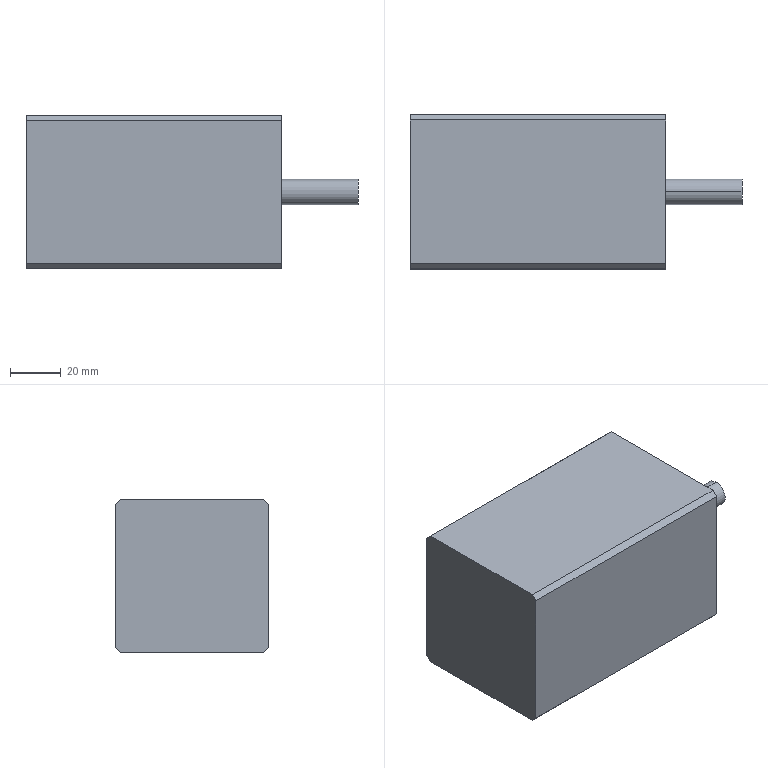Part | STEP file | Guide wheel mechanism revised.sldasm-Part-415 | 1 solid | 13 faces | box 130.5 x 60.5 x 60.5 mm | volume 369407 mm3 | plane 11 | cylinder 2 | commonest cylinder face diameters 10 x2
STEP:
#1=CARTESIAN_POINT('',(130.5,0.,5.));
#2=VERTEX_POINT('',#1);
#3=CARTESIAN_POINT('',(130.5,0.,-5.));
#4=VERTEX_POINT('',#3);
#5=CARTESIAN_POINT('',(130.5,0.,0.));
#6=DIRECTION('',(-1.,0.,0.));
#7=DIRECTION('',(0.,0.,1.));
#8=AXIS2_PLACEMENT_3D('',#5,#6,#7);
#9=CIRCLE('',#8,5.);
#10=EDGE_CURVE('',#2,#4,#9,.T.);
#11=ORIENTED_EDGE('',*,*,#10,.T.);
#12=CARTESIAN_POINT('',(100.5,0.,-5.));
#13=VERTEX_POINT('',#12);
#14=CARTESIAN_POINT('',(130.5,0.,-5.));
#15=DIRECTION('',(-1.,0.,0.));
#16=VECTOR('',#15,1000.);
#17=LINE('',#14,#16);
#18=EDGE_CURVE('',#4,#13,#17,.T.);
#19=ORIENTED_EDGE('',*,*,#18,.T.);
#20=CARTESIAN_POINT('',(100.5,0.,5.));
#21=VERTEX_POINT('',#20);
#22=CARTESIAN_POINT('',(100.5,0.,0.));
#23=DIRECTION('',(-1.,0.,0.));
#24=DIRECTION('',(0.,0.,-1.));
#25=AXIS2_PLACEMENT_3D('',#22,#23,#24);
#26=CIRCLE('',#25,5.);
#27=EDGE_CURVE('',#21,#13,#26,.T.);
#28=ORIENTED_EDGE('',*,*,#27,.F.);
#29=CARTESIAN_POINT('',(130.5,0.,5.));
#30=DIRECTION('',(-1.,0.,0.));
#31=VECTOR('',#30,1000.);
#32=LINE('',#29,#31);
#33=EDGE_CURVE('',#2,#21,#32,.T.);
#34=ORIENTED_EDGE('',*,*,#33,.F.);
#35=EDGE_LOOP('',(#11,#19,#28,#34));
#36=FACE_OUTER_BOUND('',#35,.T.);
#37=CARTESIAN_POINT('',(130.5,0.,0.));
#38=DIRECTION('',(-1.,0.,0.));
#39=DIRECTION('',(0.,0.,1.));
#40=AXIS2_PLACEMENT_3D('',#37,#38,#39);
#41=CYLINDRICAL_SURFACE('',#40,5.);
#42=ADVANCED_FACE('',(#36),#41,.T.);
#43=CARTESIAN_POINT('',(100.5,30.2,28.25));
#44=VERTEX_POINT('',#43);
#45=CARTESIAN_POINT('',(100.5,28.2,30.25));
#46=VERTEX_POINT('',#45);
#47=CARTESIAN_POINT('',(100.5,30.2,28.25));
#48=DIRECTION('',(0.,-0.7071,0.7071));
#49=VECTOR('',#48,1000.);
#50=LINE('',#47,#49);
#51=EDGE_CURVE('',#44,#46,#50,.T.);
#52=ORIENTED_EDGE('',*,*,#51,.T.);
#53=CARTESIAN_POINT('',(100.5,-28.3,30.25));
#54=VERTEX_POINT('',#53);
#55=CARTESIAN_POINT('',(100.5,28.2,30.25));
#56=DIRECTION('',(0.,-1.,0.));
#57=VECTOR('',#56,1000.);
#58=LINE('',#55,#57);
#59=EDGE_CURVE('',#46,#54,#58,.T.);
#60=ORIENTED_EDGE('',*,*,#59,.T.);
#61=CARTESIAN_POINT('',(100.5,-30.3,28.25));
#62=VERTEX_POINT('',#61);
#63=CARTESIAN_POINT('',(100.5,-28.3,30.25));
#64=DIRECTION('',(0.,-0.7071,-0.7071));
#65=VECTOR('',#64,1000.);
#66=LINE('',#63,#65);
#67=EDGE_CURVE('',#54,#62,#66,.T.);
#68=ORIENTED_EDGE('',*,*,#67,.T.);
#69=CARTESIAN_POINT('',(100.5,-30.3,-28.25));
#70=VERTEX_POINT('',#69);
#71=CARTESIAN_POINT('',(100.5,-30.3,28.25));
#72=DIRECTION('',(0.,0.,-1.));
#73=VECTOR('',#72,1000.);
#74=LINE('',#71,#73);
#75=EDGE_CURVE('',#62,#70,#74,.T.);
#76=ORIENTED_EDGE('',*,*,#75,.T.);
#77=CARTESIAN_POINT('',(100.5,-28.3,-30.25));
#78=VERTEX_POINT('',#77);
#79=CARTESIAN_POINT('',(100.5,-30.3,-28.25));
#80=DIRECTION('',(0.,0.7071,-0.7071));
#81=VECTOR('',#80,1000.);
#82=LINE('',#79,#81);
#83=EDGE_CURVE('',#70,#78,#82,.T.);
#84=ORIENTED_EDGE('',*,*,#83,.T.);
#85=CARTESIAN_POINT('',(100.5,28.2,-30.25));
#86=VERTEX_POINT('',#85);
#87=CARTESIAN_POINT('',(100.5,-28.3,-30.25));
#88=DIRECTION('',(0.,1.,0.));
#89=VECTOR('',#88,1000.);
#90=LINE('',#87,#89);
#91=EDGE_CURVE('',#78,#86,#90,.T.);
#92=ORIENTED_EDGE('',*,*,#91,.T.);
#93=CARTESIAN_POINT('',(100.5,30.2,-28.25));
#94=VERTEX_POINT('',#93);
#95=CARTESIAN_POINT('',(100.5,28.2,-30.25));
#96=DIRECTION('',(0.,0.7071,0.7071));
#97=VECTOR('',#96,1000.);
#98=LINE('',#95,#97);
#99=EDGE_CURVE('',#86,#94,#98,.T.);
#100=ORIENTED_EDGE('',*,*,#99,.T.);
#101=CARTESIAN_POINT('',(100.5,30.2,-28.25));
#102=DIRECTION('',(0.,0.,1.));
#103=VECTOR('',#102,1000.);
#104=LINE('',#101,#103);
#105=EDGE_CURVE('',#94,#44,#104,.T.);
#106=ORIENTED_EDGE('',*,*,#105,.T.);
#107=EDGE_LOOP('',(#52,#60,#68,#76,#84,#92,#100,#106));
#108=FACE_OUTER_BOUND('',#107,.T.);
#109=ORIENTED_EDGE('',*,*,#27,.T.);
#110=CARTESIAN_POINT('',(100.5,0.,0.));
#111=DIRECTION('',(-1.,0.,0.));
#112=DIRECTION('',(0.,0.,-1.));
#113=AXIS2_PLACEMENT_3D('',#110,#111,#112);
#114=CIRCLE('',#113,5.);
#115=EDGE_CURVE('',#13,#21,#114,.T.);
#116=ORIENTED_EDGE('',*,*,#115,.T.);
#117=EDGE_LOOP('',(#109,#116));
#118=FACE_BOUND('',#117,.T.);
#119=CARTESIAN_POINT('',(100.5,0.,0.));
#120=DIRECTION('',(1.,0.,0.));
#121=DIRECTION('',(0.,0.,-1.));
#122=AXIS2_PLACEMENT_3D('',#119,#120,#121);
#123=PLANE('',#122);
#124=ADVANCED_FACE('',(#108,#118),#123,.T.);
#125=CARTESIAN_POINT('',(0.,30.2,28.25));
#126=VERTEX_POINT('',#125);
#127=CARTESIAN_POINT('',(0.,28.2,30.25));
#128=VERTEX_POINT('',#127);
#129=CARTESIAN_POINT('',(0.,30.2,28.25));
#130=DIRECTION('',(0.,-0.7071,0.7071));
#131=VECTOR('',#130,1000.);
#132=LINE('',#129,#131);
#133=EDGE_CURVE('',#126,#128,#132,.T.);
#134=ORIENTED_EDGE('',*,*,#133,.T.);
#135=CARTESIAN_POINT('',(100.5,28.2,30.25));
#136=DIRECTION('',(-1.,0.,0.));
#137=VECTOR('',#136,1000.);
#138=LINE('',#135,#137);
#139=EDGE_CURVE('',#46,#128,#138,.T.);
#140=ORIENTED_EDGE('',*,*,#139,.F.);
#141=ORIENTED_EDGE('',*,*,#51,.F.);
#142=CARTESIAN_POINT('',(100.5,30.2,28.25));
#143=DIRECTION('',(-1.,0.,0.));
#144=VECTOR('',#143,1000.);
#145=LINE('',#142,#144);
#146=EDGE_CURVE('',#44,#126,#145,.T.);
#147=ORIENTED_EDGE('',*,*,#146,.T.);
#148=EDGE_LOOP('',(#134,#140,#141,#147));
#149=FACE_OUTER_BOUND('',#148,.T.);
#150=CARTESIAN_POINT('',(100.5,30.2,28.25));
#151=DIRECTION('',(0.,-0.7071,-0.7071));
#152=DIRECTION('',(0.,0.7071,-0.7071));
#153=AXIS2_PLACEMENT_3D('',#150,#151,#152);
#154=PLANE('',#153);
#155=ADVANCED_FACE('',(#149),#154,.F.);
#156=CARTESIAN_POINT('',(0.,-28.3,30.25));
#157=VERTEX_POINT('',#156);
#158=CARTESIAN_POINT('',(0.,28.2,30.25));
#159=DIRECTION('',(0.,-1.,0.));
#160=VECTOR('',#159,1000.);
#161=LINE('',#158,#160);
#162=EDGE_CURVE('',#128,#157,#161,.T.);
#163=ORIENTED_EDGE('',*,*,#162,.T.);
#164=CARTESIAN_POINT('',(100.5,-28.3,30.25));
#165=DIRECTION('',(-1.,0.,0.));
#166=VECTOR('',#165,1000.);
#167=LINE('',#164,#166);
#168=EDGE_CURVE('',#54,#157,#167,.T.);
#169=ORIENTED_EDGE('',*,*,#168,.F.);
#170=ORIENTED_EDGE('',*,*,#59,.F.);
#171=ORIENTED_EDGE('',*,*,#139,.T.);
#172=EDGE_LOOP('',(#163,#169,#170,#171));
#173=FACE_OUTER_BOUND('',#172,.T.);
#174=CARTESIAN_POINT('',(100.5,28.2,30.25));
#175=DIRECTION('',(0.,0.,-1.));
#176=DIRECTION('',(-1.,0.,0.));
#177=AXIS2_PLACEMENT_3D('',#174,#175,#176);
#178=PLANE('',#177);
#179=ADVANCED_FACE('',(#173),#178,.F.);
#180=CARTESIAN_POINT('',(0.,-30.3,28.25));
#181=VERTEX_POINT('',#180);
#182=CARTESIAN_POINT('',(0.,-28.3,30.25));
#183=DIRECTION('',(0.,-0.7071,-0.7071));
#184=VECTOR('',#183,1000.);
#185=LINE('',#182,#184);
#186=EDGE_CURVE('',#157,#181,#185,.T.);
#187=ORIENTED_EDGE('',*,*,#186,.T.);
#188=CARTESIAN_POINT('',(100.5,-30.3,28.25));
#189=DIRECTION('',(-1.,0.,0.));
#190=VECTOR('',#189,1000.);
#191=LINE('',#188,#190);
#192=EDGE_CURVE('',#62,#181,#191,.T.);
#193=ORIENTED_EDGE('',*,*,#192,.F.);
#194=ORIENTED_EDGE('',*,*,#67,.F.);
#195=ORIENTED_EDGE('',*,*,#168,.T.);
#196=EDGE_LOOP('',(#187,#193,#194,#195));
#197=FACE_OUTER_BOUND('',#196,.T.);
#198=CARTESIAN_POINT('',(100.5,-28.3,30.25));
#199=DIRECTION('',(0.,0.7071,-0.7071));
#200=DIRECTION('',(0.,0.7071,0.7071));
#201=AXIS2_PLACEMENT_3D('',#198,#199,#200);
#202=PLANE('',#201);
#203=ADVANCED_FACE('',(#197),#202,.F.);
#204=CARTESIAN_POINT('',(0.,-30.3,-28.25));
#205=VERTEX_POINT('',#204);
#206=CARTESIAN_POINT('',(0.,-30.3,28.25));
#207=DIRECTION('',(0.,0.,-1.));
#208=VECTOR('',#207,1000.);
#209=LINE('',#206,#208);
#210=EDGE_CURVE('',#181,#205,#209,.T.);
#211=ORIENTED_EDGE('',*,*,#210,.T.);
#212=CARTESIAN_POINT('',(100.5,-30.3,-28.25));
#213=DIRECTION('',(-1.,0.,0.));
#214=VECTOR('',#213,1000.);
#215=LINE('',#212,#214);
#216=EDGE_CURVE('',#70,#205,#215,.T.);
#217=ORIENTED_EDGE('',*,*,#216,.F.);
#218=ORIENTED_EDGE('',*,*,#75,.F.);
#219=ORIENTED_EDGE('',*,*,#192,.T.);
#220=EDGE_LOOP('',(#211,#217,#218,#219));
#221=FACE_OUTER_BOUND('',#220,.T.);
#222=CARTESIAN_POINT('',(100.5,-30.3,28.25));
#223=DIRECTION('',(0.,1.,0.));
#224=DIRECTION('',(0.,0.,1.));
#225=AXIS2_PLACEMENT_3D('',#222,#223,#224);
#226=PLANE('',#225);
#227=ADVANCED_FACE('',(#221),#226,.F.);
#228=CARTESIAN_POINT('',(0.,-28.3,-30.25));
#229=VERTEX_POINT('',#228);
#230=CARTESIAN_POINT('',(0.,-30.3,-28.25));
#231=DIRECTION('',(0.,0.7071,-0.7071));
#232=VECTOR('',#231,1000.);
#233=LINE('',#230,#232);
#234=EDGE_CURVE('',#205,#229,#233,.T.);
#235=ORIENTED_EDGE('',*,*,#234,.T.);
#236=CARTESIAN_POINT('',(100.5,-28.3,-30.25));
#237=DIRECTION('',(-1.,0.,0.));
#238=VECTOR('',#237,1000.);
#239=LINE('',#236,#238);
#240=EDGE_CURVE('',#78,#229,#239,.T.);
#241=ORIENTED_EDGE('',*,*,#240,.F.);
#242=ORIENTED_EDGE('',*,*,#83,.F.);
#243=ORIENTED_EDGE('',*,*,#216,.T.);
#244=EDGE_LOOP('',(#235,#241,#242,#243));
#245=FACE_OUTER_BOUND('',#244,.T.);
#246=CARTESIAN_POINT('',(100.5,-30.3,-28.25));
#247=DIRECTION('',(0.,0.7071,0.7071));
#248=DIRECTION('',(0.,-0.7071,0.7071));
#249=AXIS2_PLACEMENT_3D('',#246,#247,#248);
#250=PLANE('',#249);
#251=ADVANCED_FACE('',(#245),#250,.F.);
#252=CARTESIAN_POINT('',(0.,28.2,-30.25));
#253=VERTEX_POINT('',#252);
#254=CARTESIAN_POINT('',(0.,-28.3,-30.25));
#255=DIRECTION('',(0.,1.,0.));
#256=VECTOR('',#255,1000.);
#257=LINE('',#254,#256);
#258=EDGE_CURVE('',#229,#253,#257,.T.);
#259=ORIENTED_EDGE('',*,*,#258,.T.);
#260=CARTESIAN_POINT('',(100.5,28.2,-30.25));
#261=DIRECTION('',(-1.,0.,0.));
#262=VECTOR('',#261,1000.);
#263=LINE('',#260,#262);
#264=EDGE_CURVE('',#86,#253,#263,.T.);
#265=ORIENTED_EDGE('',*,*,#264,.F.);
#266=ORIENTED_EDGE('',*,*,#91,.F.);
#267=ORIENTED_EDGE('',*,*,#240,.T.);
#268=EDGE_LOOP('',(#259,#265,#266,#267));
#269=FACE_OUTER_BOUND('',#268,.T.);
#270=CARTESIAN_POINT('',(100.5,-28.3,-30.25));
#271=DIRECTION('',(0.,0.,1.));
#272=DIRECTION('',(1.,0.,0.));
#273=AXIS2_PLACEMENT_3D('',#270,#271,#272);
#274=PLANE('',#273);
#275=ADVANCED_FACE('',(#269),#274,.F.);
#276=CARTESIAN_POINT('',(0.,30.2,-28.25));
#277=VERTEX_POINT('',#276);
#278=CARTESIAN_POINT('',(0.,28.2,-30.25));
#279=DIRECTION('',(0.,0.7071,0.7071));
#280=VECTOR('',#279,1000.);
#281=LINE('',#278,#280);
#282=EDGE_CURVE('',#253,#277,#281,.T.);
#283=ORIENTED_EDGE('',*,*,#282,.T.);
#284=CARTESIAN_POINT('',(100.5,30.2,-28.25));
#285=DIRECTION('',(-1.,0.,0.));
#286=VECTOR('',#285,1000.);
#287=LINE('',#284,#286);
#288=EDGE_CURVE('',#94,#277,#287,.T.);
#289=ORIENTED_EDGE('',*,*,#288,.F.);
#290=ORIENTED_EDGE('',*,*,#99,.F.);
#291=ORIENTED_EDGE('',*,*,#264,.T.);
#292=EDGE_LOOP('',(#283,#289,#290,#291));
#293=FACE_OUTER_BOUND('',#292,.T.);
#294=CARTESIAN_POINT('',(100.5,28.2,-30.25));
#295=DIRECTION('',(0.,-0.7071,0.7071));
#296=DIRECTION('',(0.,-0.7071,-0.7071));
#297=AXIS2_PLACEMENT_3D('',#294,#295,#296);
#298=PLANE('',#297);
#299=ADVANCED_FACE('',(#293),#298,.F.);
#300=CARTESIAN_POINT('',(0.,30.2,-28.25));
#301=DIRECTION('',(0.,0.,1.));
#302=VECTOR('',#301,1000.);
#303=LINE('',#300,#302);
#304=EDGE_CURVE('',#277,#126,#303,.T.);
#305=ORIENTED_EDGE('',*,*,#304,.T.);
#306=ORIENTED_EDGE('',*,*,#146,.F.);
#307=ORIENTED_EDGE('',*,*,#105,.F.);
#308=ORIENTED_EDGE('',*,*,#288,.T.);
#309=EDGE_LOOP('',(#305,#306,#307,#308));
#310=FACE_OUTER_BOUND('',#309,.T.);
#311=CARTESIAN_POINT('',(100.5,30.2,-28.25));
#312=DIRECTION('',(0.,-1.,0.));
#313=DIRECTION('',(0.,0.,-1.));
#314=AXIS2_PLACEMENT_3D('',#311,#312,#313);
#315=PLANE('',#314);
#316=ADVANCED_FACE('',(#310),#315,.F.);
#317=ORIENTED_EDGE('',*,*,#133,.F.);
#318=ORIENTED_EDGE('',*,*,#304,.F.);
#319=ORIENTED_EDGE('',*,*,#282,.F.);
#320=ORIENTED_EDGE('',*,*,#258,.F.);
#321=ORIENTED_EDGE('',*,*,#234,.F.);
#322=ORIENTED_EDGE('',*,*,#210,.F.);
#323=ORIENTED_EDGE('',*,*,#186,.F.);
#324=ORIENTED_EDGE('',*,*,#162,.F.);
#325=EDGE_LOOP('',(#317,#318,#319,#320,#321,#322,#323,#324));
#326=FACE_OUTER_BOUND('',#325,.T.);
#327=CARTESIAN_POINT('',(0.,0.,0.));
#328=DIRECTION('',(1.,0.,0.));
#329=DIRECTION('',(0.,0.,-1.));
#330=AXIS2_PLACEMENT_3D('',#327,#328,#329);
#331=PLANE('',#330);
#332=ADVANCED_FACE('',(#326),#331,.F.);
#333=ORIENTED_EDGE('',*,*,#18,.F.);
#334=CARTESIAN_POINT('',(130.5,0.,0.));
#335=DIRECTION('',(-1.,0.,0.));
#336=DIRECTION('',(0.,0.,1.));
#337=AXIS2_PLACEMENT_3D('',#334,#335,#336);
#338=CIRCLE('',#337,5.);
#339=EDGE_CURVE('',#4,#2,#338,.T.);
#340=ORIENTED_EDGE('',*,*,#339,.T.);
#341=ORIENTED_EDGE('',*,*,#33,.T.);
#342=ORIENTED_EDGE('',*,*,#115,.F.);
#343=EDGE_LOOP('',(#333,#340,#341,#342));
#344=FACE_OUTER_BOUND('',#343,.T.);
#345=CARTESIAN_POINT('',(130.5,0.,0.));
#346=DIRECTION('',(-1.,0.,0.));
#347=DIRECTION('',(0.,0.,1.));
#348=AXIS2_PLACEMENT_3D('',#345,#346,#347);
#349=CYLINDRICAL_SURFACE('',#348,5.);
#350=ADVANCED_FACE('',(#344),#349,.T.);
#351=ORIENTED_EDGE('',*,*,#10,.F.);
#352=ORIENTED_EDGE('',*,*,#339,.F.);
#353=EDGE_LOOP('',(#351,#352));
#354=FACE_OUTER_BOUND('',#353,.T.);
#355=CARTESIAN_POINT('',(130.5,5.,0.));
#356=DIRECTION('',(-1.,0.,0.));
#357=DIRECTION('',(0.,0.,1.));
#358=AXIS2_PLACEMENT_3D('',#355,#356,#357);
#359=PLANE('',#358);
#360=ADVANCED_FACE('',(#354),#359,.F.);
#361=CLOSED_SHELL('',(#42,#124,#155,#179,#203,#227,#251,#275,#299,#316,#332,#350,#360));
#362=MANIFOLD_SOLID_BREP('',#361);
#363=CARTESIAN_POINT('',(0.,0.,0.));
#364=DIRECTION('',(0.,0.,1.));
#365=DIRECTION('',(1.,0.,0.));
#366=AXIS2_PLACEMENT_3D('',#363,#364,#365);
#367=(LENGTH_UNIT()NAMED_UNIT(*)SI_UNIT(.MILLI.,.METRE.));
#368=UNCERTAINTY_MEASURE_WITH_UNIT(LENGTH_MEASURE(0.00001),#367,'','');
#369=(NAMED_UNIT(*)PLANE_ANGLE_UNIT()SI_UNIT($,.RADIAN.));
#370=(NAMED_UNIT(*)SI_UNIT($,.STERADIAN.)SOLID_ANGLE_UNIT());
#371=(GEOMETRIC_REPRESENTATION_CONTEXT(3)GLOBAL_UNCERTAINTY_ASSIGNED_CONTEXT((#368))GLOBAL_UNIT_ASSIGNED_CONTEXT((#367,#369,#370))REPRESENTATION_CONTEXT('',''));
#372=ADVANCED_BREP_SHAPE_REPRESENTATION('',(#362,#366),#371);